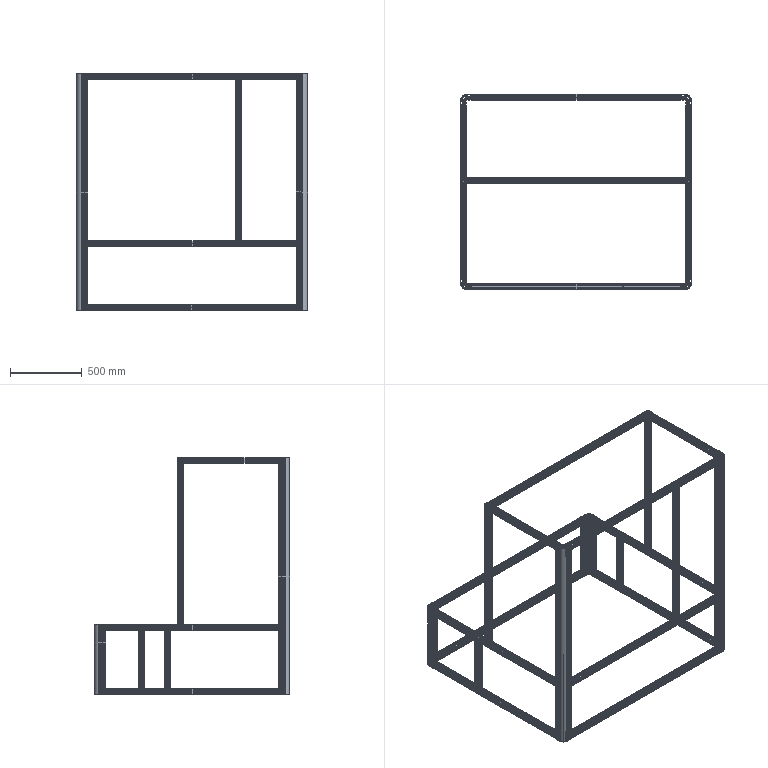Part | 29 solids | 3084 faces | volume 18019201 mm3 | plane 2542 | cylinder 542 | commonest cylinder face diameters 6.8 x176 8.2 x130 5 x112 9 x112 66.41 x4 76.531 x4